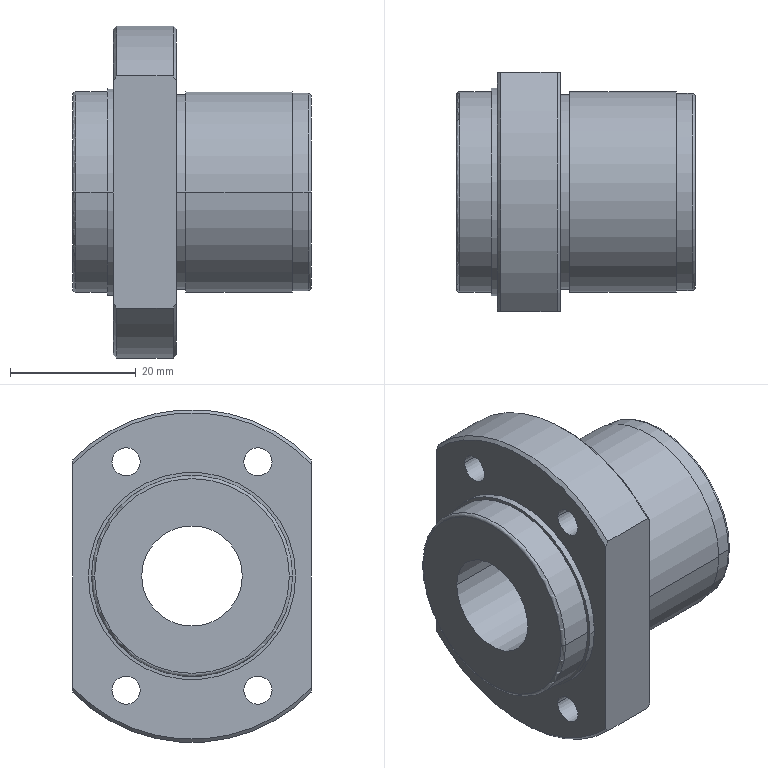Part | STEP file | Screw nut BLK1616-3.6G | 1 solid | 39 faces | box 38 x 38 x 53 mm | volume 32346 mm3 | cylinder 22 | plane 9 | torus 4 | cone 4 | commonest cylinder face diameters 4.5 x8 32 x4 16 x2 31 x2 31.4 x2 33 x2